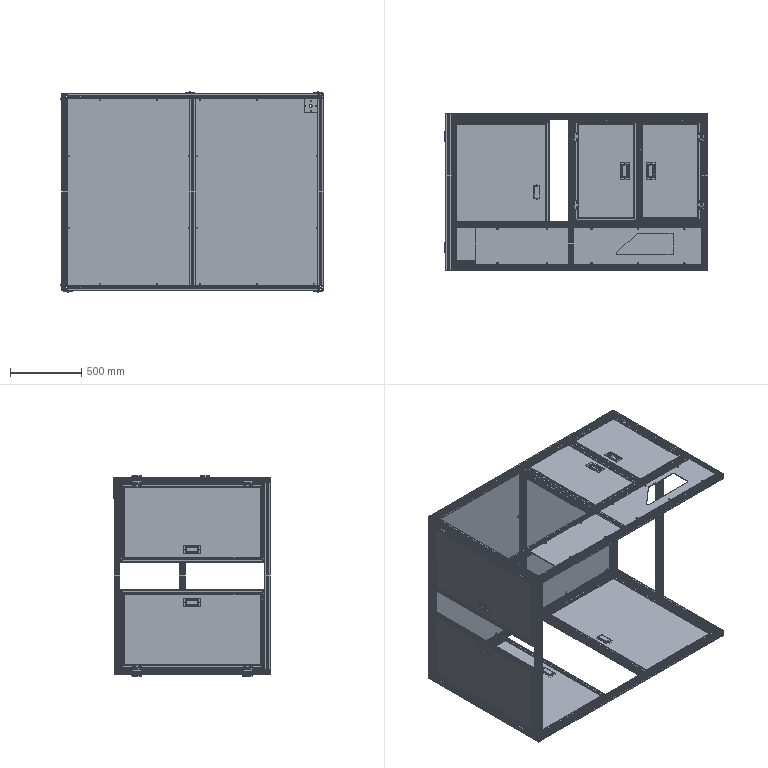Part | SolidWorks | 70 solids | 3342 faces | volume 51712509 mm3 | plane 1942 | cylinder 1082 | cone 270 | sphere 48 | commonest cylinder face diameters 5 x168 19 x133 2 x120 8 x112 10 x100 4 x72